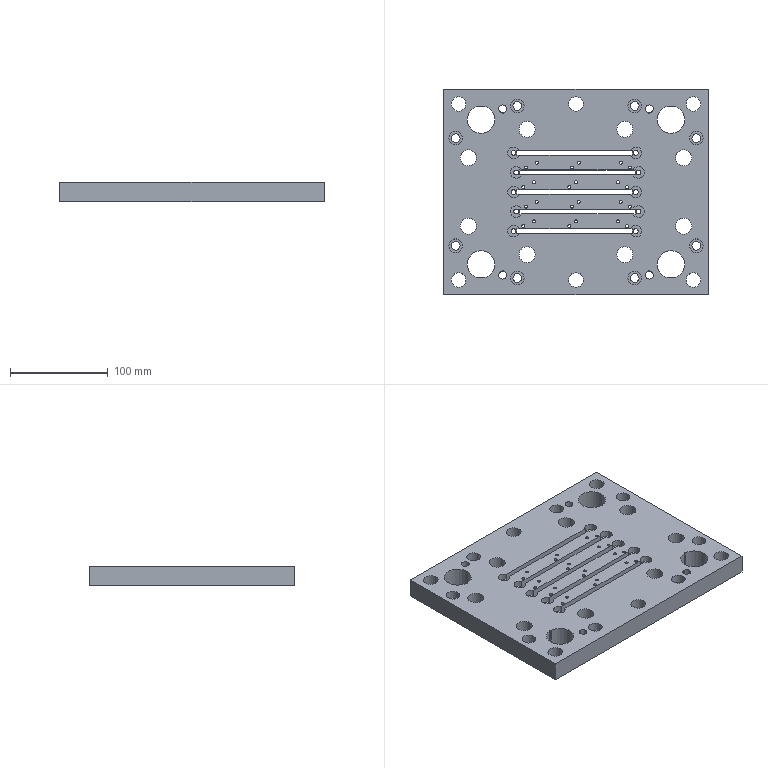Part | STEP file | 1 solid | 163 faces | box 270 x 210 x 20 mm | volume 936503 mm3 | cylinder 106 | plane 44 | cone 13 | commonest cylinder face diameters 1 x24 3.1 x24 5 x10 12 x10 9 x8 14 x8